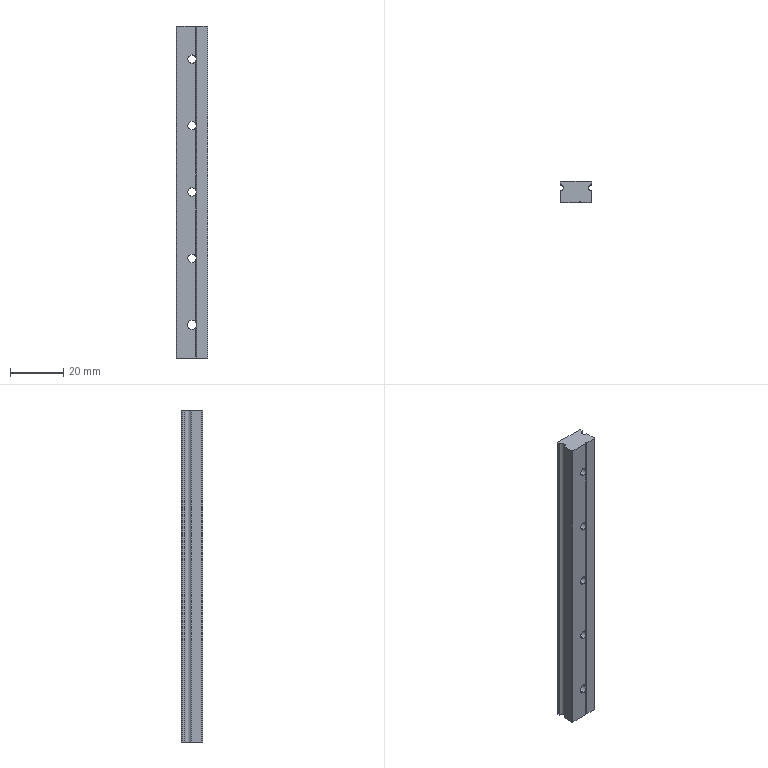Part | STEP file | Bag feed mounting electronic clip MGN12C (slide rail) Z-axis | 1 solid | 42 faces | box 12 x 8 x 125 mm | volume 10672 mm3 | cylinder 24 | plane 18 | commonest cylinder face diameters 6 x10 3.2 x8 2.5 x3 3.5 x2 0.6 x1